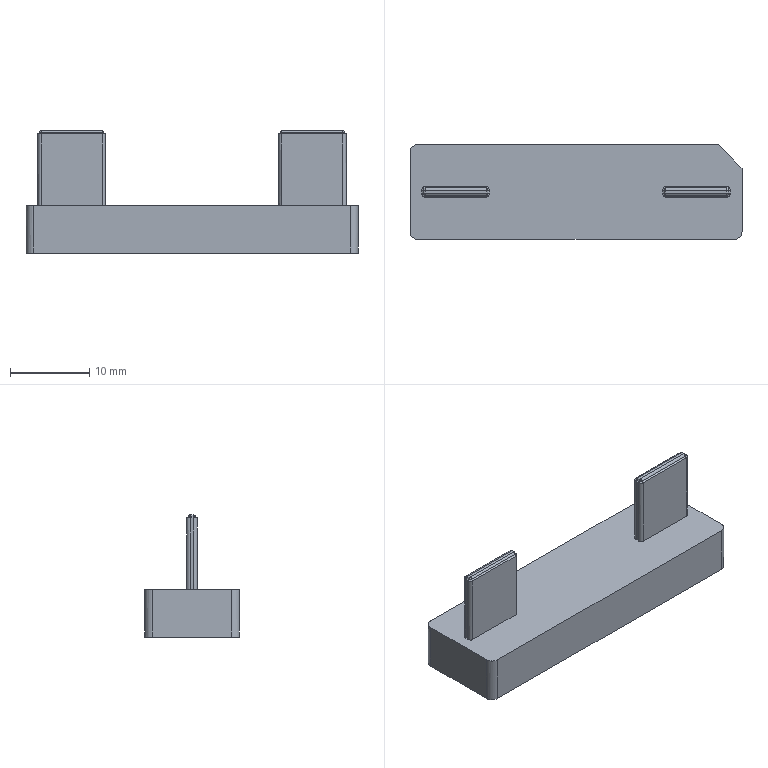NC program | PowerMill | posted with a generic post | part box 42 x 12 x 15.447 mm
Lines 10041 to 10905 of 88764:
N10138 M6
N10139 S18000 M03
N10140 G00 G90 X0.0 Y0.0
N10141 G43 Z10.797 H14
N10142
N10143 G05 P10000 R8
N10144 X20.3526 Y-2.564
N10145 Z0.922
N10146 G01 Z-0.278 F1200.0
N10147 X20.3332 Y-2.4952 F2000.0
N10148 X20.3063 Y-2.4291
N10149 X20.2722 Y-2.3663
N10150 X20.2313 Y-2.3077
N10151 X20.1841 Y-2.254
N10152 X20.1312 Y-2.2059
N10153 X20.0734 Y-2.1641
N10154 X20.0112 Y-2.1289
N10155 X19.9455 Y-2.1009
N10156 X19.877 Y-2.0804
N10157 X19.8067 Y-2.0676
N10158 X19.7354 Y-2.0628
N10159 X19.664 Y-2.0659
N10160 X19.5935 Y-2.077
N10161 X19.589 Y-2.078
N10162 X19.4691 Y-2.1046
N10163 X19.3617 Y-2.1219
N10164 X19.24 Y-2.1338
N10165 X19.1048 Y-2.1394
N10166 X18.6048 Y-2.1399
N10167 X18.1048
N10168 X17.6048 Y-2.14
N10169 X17.1048
N10170 X16.6048
N10171 X16.1048
N10172 X15.6048 Y-2.1399
N10173 X15.1129
N10174 X14.621
N10175 X14.1292
N10176 X13.6374 Y-2.14
N10177 X13.1456 Y-2.1401
N10178 X12.6538
N10179 X12.162 Y-2.1403
N10180 X11.6702 Y-2.1406
N10181 X11.4289 Y-2.1408
N10182 X11.2906 Y-2.1373
N10183 X11.1595 Y-2.1265
N10184 X11.0349 Y-2.1087
N10185 X10.9163 Y-2.0842
N10186 X10.8016 Y-2.0527
N10187 X10.6821 Y-2.0117
N10188 X10.5659 Y-1.9634
N10189 X10.4536 Y-1.9081
N10190 X10.3455 Y-1.846
N10191 X10.242 Y-1.7775
N10192 X10.1435 Y-1.7027
N10193 X10.0489 Y-1.6211
N10194 X9.96 Y-1.5341
N10195 X9.8771 Y-1.4418
N10196 X9.8 Y-1.3442
N10197 X9.7288 Y-1.2412
N10198 X9.6636 Y-1.1327
N10199 X9.6043 Y-1.0189
N10200 X9.5539 Y-0.906
N10201 X9.512 Y-0.7933
N10202 X9.4784 Y-0.6813
N10203 X9.4571 Y-0.5918
N10204 X9.4387 Y-0.5016
N10205 X9.4242 Y-0.4109
N10206 X9.4151 Y-0.3193
N10207 X9.4113 Y-0.2272
N10208 X9.4118 Y0.2682
N10209 X9.4163 Y0.3659
N10210 X9.4284 Y0.463
N10211 X9.445 Y0.5596
N10212 X9.4639 Y0.6555
N10213 X9.4927 Y0.764
N10214 X9.5308 Y0.8775
N10215 X9.5775 Y0.9928
N10216 X9.6318 Y1.1063
N10217 X9.6916 Y1.2136
N10218 X9.7586 Y1.3178
N10219 X9.8334 Y1.4194
N10220 X9.9148 Y1.5169
N10221 X10.0011 Y1.6081
N10222 X10.0918 Y1.6926
N10223 X10.187 Y1.7705
N10224 X10.2875 Y1.8424
N10225 X10.3927 Y1.9078
N10226 X10.5022 Y1.9666
N10227 X10.6156 Y2.0184
N10228 X10.7325 Y2.0629
N10229 X10.8518 Y2.0999
N10230 X10.961 Y2.1271
N10231 X11.0715 Y2.1479
N10232 X11.1832 Y2.1622
N10233 X11.3088 Y2.1706
N10234 X11.4243 Y2.1728
N10235 X11.9156
N10236 X12.4068
N10237 X12.8979
N10238 X13.3891
N10239 X13.8803
N10240 X14.3714
N10241 X14.8625
N10242 X15.3536 Y2.1727
N10243 X15.8446
N10244 X16.3357
N10245 X16.8267 Y2.1728
N10246 X17.3177 Y2.173
N10247 X17.8086 Y2.1731
N10248 X18.2995 Y2.1733
N10249 X18.7904 Y2.1736
N10250 X19.0484 Y2.1738
N10251 X19.1858 Y2.1703
N10252 X19.3171 Y2.1595
N10253 X19.4429 Y2.1415
N10254 X19.564 Y2.1164
N10255 X19.6819 Y2.0841
N10256 X19.7976 Y2.0442
N10257 X19.9139 Y1.9957
N10258 X20.0265 Y1.9401
N10259 X20.135 Y1.8777
N10260 X20.2389 Y1.8088
N10261 X20.3377 Y1.7337
N10262 X20.4314 Y1.6525
N10263 X20.5198 Y1.5655
N10264 X20.6038 Y1.4717
N10265 X20.682 Y1.3724
N10266 X20.7542 Y1.2679
N10267 X20.8199 Y1.1586
N10268 X20.8774 Y1.0478
N10269 X20.9282 Y0.9327
N10270 X20.9712 Y0.8154
N10271 X21.0062 Y0.6975
N10272 X21.0329 Y0.5802
N10273 X21.0526 Y0.4631
N10274 X21.0649 Y0.3501
N10275 X21.0694 Y0.2422
N10276 X21.0688 Y-0.1885
N10277 X21.0671 Y-0.2921
N10278 X21.0583 Y-0.3984
N10279 X21.0412 Y-0.5104
N10280 X21.0152 Y-0.6295
N10281 X20.9813 Y-0.751
N10282 X20.9401 Y-0.8698
N10283 X20.8914 Y-0.9858
N10284 X20.8355 Y-1.0985
N10285 X20.7726 Y-1.2075
N10286 X20.7028 Y-1.3124
N10287 X20.6264 Y-1.4127
N10288 X20.5438 Y-1.508
N10289 X20.4553 Y-1.5979
N10290 X20.3612 Y-1.6823
N10291 X20.2716 Y-1.7533
N10292 X20.1752 Y-1.8204
N10293 X20.0699 Y-1.8843
N10294 X19.9577 Y-1.9432
N10295 X19.8435 Y-1.9943
N10296 X19.7306 Y-2.0366
N10297 X19.6212 Y-2.0697
N10298 X19.589 Y-2.078
N10299 X19.4894 Y-2.1004
N10300 X19.3889 Y-2.1184
N10301 X19.2669 Y-2.1323 Z-0.2781
N10302 X19.1358 Y-2.1395
N10303 X18.6358 Y-2.1409 Z-0.2783
N10304 X18.1358 Y-2.1418 Z-0.2785
N10305 X17.6358 Y-2.143 Z-0.2787
N10306 X17.1358 Y-2.144 Z-0.2789
N10307 X16.6358 Y-2.1447 Z-0.2791
N10308 X16.1358 Y-2.1455 Z-0.2792
N10309 X15.6358 Y-2.1463 Z-0.2794
N10310 X15.1404 Y-2.147 Z-0.2796
N10311 X14.645 Y-2.1478 Z-0.2797
N10312 X14.1497 Y-2.1485 Z-0.2799
N10313 X13.6544 Y-2.1493 Z-0.28
N10314 X13.159 Y-2.1499 Z-0.2802
N10315 X12.6637 Y-2.1504 Z-0.2803
N10316 X12.1684 Y-2.1509 Z-0.2805
N10317 X11.6731 Y-2.152 Z-0.2806
N10318 X11.4289 Y-2.1529
N10319 X11.2951 Y-2.1498
N10320 X11.1628 Y-2.1395
N10321 X11.036 Y-2.1221
N10322 X10.9166 Y-2.0983
N10323 X10.8055 Y-2.0686 Z-0.2805
N10324 X10.7001 Y-2.0329
N10325 X10.5823 Y-1.9857
N10326 X10.4757 Y-1.9353 Z-0.2804
N10327 X10.3828 Y-1.8839
N10328 X10.298 Y-1.8316 Z-0.2805
N10329 X10.216 Y-1.7752 Z-0.2807
N10330 X10.1372 Y-1.7143 Z-0.2808
N10331 X10.0407 Y-1.6308
N10332 X9.9501 Y-1.5419 Z-0.2809
N10333 X9.8659 Y-1.4484
N10334 X9.7887 Y-1.3508 Z-0.281
N10335 X9.7188 Y-1.2497
N10336 X9.6619 Y-1.1563 Z-0.2811
N10337 X9.6029 Y-1.0465 Z-0.2813
N10338 X9.557 Y-0.9473 Z-0.2814
N10339 X9.5184 Y-0.849
N10340 X9.4776 Y-0.726
N10341 X9.445 Y-0.6031 Z-0.2815
N10342 X9.421 Y-0.484
N10343 X9.4057 Y-0.3706 Z-0.2816
N10344 X9.3985 Y-0.2638 Z-0.2817
N10345 X9.3962 Y0.2357
N10346 X9.4001 Y0.3396
N10347 X9.4107 Y0.4458 Z-0.2818
N10348 X9.4295 Y0.5633
N10349 X9.4573 Y0.689 Z-0.2819
N10350 X9.491 Y0.8076
N10351 X9.5278 Y0.9131 Z-0.282
N10352 X9.5699 Y1.0142
N10353 X9.6257 Y1.1291 Z-0.2819
N10354 X9.6896 Y1.2428
N10355 X9.7491 Y1.3348
N10356 X9.8198 Y1.4301
N10357 X9.8874 Y1.5125
N10358 X9.9581 Y1.5897 Z-0.282
N10359 X10.041 Y1.6703 Z-0.2823
N10360 X10.1199 Y1.7393 Z-0.2824
N10361 X10.2022 Y1.804
N10362 X10.3047 Y1.8752
N10363 X10.4118 Y1.94
N10364 X10.5233 Y1.998
N10365 X10.6388 Y2.0491 Z-0.2825
N10366 X10.7579 Y2.0931
N10367 X10.8801 Y2.13
N10368 X10.9978 Y2.1578
N10369 X11.1109 Y2.1769
N10370 X11.2202 Y2.1878
N10371 X11.3491 Y2.193 Z-0.2829
N10372 X11.8464 Y2.1942 Z-0.2833
N10373 X12.3437 Y2.195 Z-0.2835
N10374 X12.841 Y2.1958 Z-0.2836
N10375 X13.3383 Y2.1965 Z-0.2838
N10376 X13.8355 Y2.1971 Z-0.284
N10377 X14.3327 Y2.1977 Z-0.2841
N10378 X14.8299 Y2.1984 Z-0.2843
N10379 X15.3271 Y2.1992 Z-0.2845
N10380 X15.8242 Y2.1999 Z-0.2847
N10381 X16.3213 Y2.2006 Z-0.2849
N10382 X16.8184 Y2.2013 Z-0.2851
N10383 X17.3154 Y2.202 Z-0.2853
N10384 X17.8125 Y2.2028 Z-0.2854
N10385 X18.3095 Y2.2036 Z-0.2856
N10386 X18.8064 Y2.2045 Z-0.2857
N10387 X18.9732 Y2.2049
N10388 X19.0454 Y2.2051
N10389 X19.1176 Y2.2052
N10390 X19.1898 Y2.2044
N10391 X19.2619 Y2.2001 Z-0.2858
N10392 X19.3336 Y2.192
N10393 X19.4051 Y2.1823
N10394 X19.5208 Y2.161
N10395 X19.6387 Y2.1313
N10396 X19.7585 Y2.093 Z-0.2859
N10397 X19.8778 Y2.0469
N10398 X19.9912 Y1.9948 Z-0.286
N10399 X20.0927 Y1.9404 Z-0.2861
N10400 X20.1909 Y1.8799
N10401 X20.2937 Y1.8079 Z-0.2862
N10402 X20.3919 Y1.7299
N10403 X20.4781 Y1.6525 Z-0.2863
N10404 X20.5587 Y1.5703
N10405 X20.6421 Y1.4745 Z-0.2864
N10406 X20.7193 Y1.3737
N10407 X20.7903 Y1.2679 Z-0.2865
N10408 X20.8553 Y1.1568
N10409 X20.9089 Y1.0516 Z-0.2866
N10410 X20.9561 Y0.9435 Z-0.2867
N10411 X20.9974 Y0.8291
N10412 X21.033 Y0.7076 Z-0.2868
N10413 X21.0627 Y0.5782
N10414 X21.0809 Y0.4686 Z-0.2869
N10415 X21.0932 Y0.3479
N10416 X21.0999 Y0.2097
N10417 X21.1011 Y0.0391 Z-0.287
N10418 X21.099 Y-0.1874 Z-0.2871
N10419 X21.0979 Y-0.2647
N10420 X21.0938 Y-0.3419
N10421 X21.0852 Y-0.4187 Z-0.2872
N10422 X21.0722 Y-0.4951
N10423 X21.0582 Y-0.5712
N10424 X21.0426 Y-0.647
N10425 X21.016 Y-0.7433 Z-0.2873
N10426 X20.9761 Y-0.8621
N10427 X20.9295 Y-0.9782 Z-0.2874
N10428 X20.8754 Y-1.0917
N10429 X20.8135 Y-1.2028 Z-0.2875
N10430 X20.7439 Y-1.3117
N10431 X20.6749 Y-1.4071
N10432 X20.5994 Y-1.4987 Z-0.2876
N10433 X20.5146 Y-1.5895
N10434 X20.4278 Y-1.6724 Z-0.2877
N10435 X20.3357 Y-1.7504
N10436 X20.2363 Y-1.8241 Z-0.2878
N10437 X20.1306 Y-1.8927
N10438 X20.0198 Y-1.9551
N10439 X19.9058 Y-2.0102 Z-0.2879
N10440 X19.7907 Y-2.0571
N10441 X19.676 Y-2.0957 Z-0.288
N10442 X19.5985 Y-2.1172
N10443 X19.4951 Y-2.1417
N10444 X19.3904 Y-2.1599 Z-0.2881
N10445 X19.2848 Y-2.1724
N10446 X19.1751 Y-2.1792
N10447 X19.0483 Y-2.181 Z-0.2882
N10448 X18.5483 Y-2.1813 Z-0.2884
N10449 X18.0483 Y-2.1817 Z-0.2885
N10450 X17.5483 Y-2.1822 Z-0.2887
N10451 X17.0483 Y-2.1827 Z-0.2889
N10452 X16.5483 Y-2.1833 Z-0.2891
N10453 X16.0483 Y-2.1838 Z-0.2892
N10454 X15.5483 Y-2.1843 Z-0.2894
N10455 X15.0513 Y-2.1847 Z-0.2896
N10456 X14.5543 Y-2.1851 Z-0.2897
N10457 X14.0573 Y-2.1855 Z-0.2899
N10458 X13.5603 Y-2.186 Z-0.2901
N10459 X13.0633 Y-2.1864 Z-0.2903
N10460 X12.5664 Y-2.1868 Z-0.2904
N10461 X12.0694 Y-2.1873 Z-0.2906
N10462 X11.5725 Y-2.1882 Z-0.2908
N10463 X11.4272 Y-2.1886
N10464 X11.2915 Y-2.1859 Z-0.2909
N10465 X11.1735 Y-2.1771
N10466 X11.0592 Y-2.1618 Z-0.291
N10467 X10.9327 Y-2.1378
N10468 X10.8127 Y-2.1073 Z-0.2911
N10469 X10.6978 Y-2.0702
N10470 X10.5846 Y-2.0253
N10471 X10.4719 Y-1.9722
N10472 X10.3609 Y-1.911 Z-0.2912
N10473 X10.2533 Y-1.8426
N10474 X10.151 Y-1.7683 Z-0.2913
N10475 X10.0553 Y-1.6891 Z-0.2914
N10476 X9.9672 Y-1.6061
N10477 X9.8858 Y-1.5197
N10478 X9.8093 Y-1.429 Z-0.2915
N10479 X9.7382 Y-1.334
N10480 X9.6691 Y-1.2288 Z-0.2916
N10481 X9.6073 Y-1.1204
N10482 X9.5525 Y-1.0084
N10483 X9.5032 Y-0.8897 Z-0.2917
N10484 X9.4607 Y-0.7666
N10485 X9.4282 Y-0.6512 Z-0.2918
N10486 X9.4029 Y-0.5334
N10487 X9.3844 Y-0.4103 Z-0.2919
N10488 X9.3731 Y-0.2816
N10489 X9.3691 Y-0.1469 Z-0.292
N10490 X9.3699 Y-0.0057
N10491 X9.3684 Y0.1655 Z-0.2921
N10492 X9.3687 Y0.2557
N10493 X9.3738 Y0.3457
N10494 X9.3784 Y0.3887
N10495 X9.3834 Y0.4317 Z-0.2922
N10496 X9.3918 Y0.4976
N10497 X9.398 Y0.5404
N10498 X9.4057 Y0.5829
N10499 X9.4254 Y0.6742
N10500 X9.4459 Y0.7514 Z-0.2923
N10501 X9.485 Y0.876
N10502 X9.528 Y0.9893 Z-0.2924
N10503 X9.5768 Y1.0968
N10504 X9.6364 Y1.2091
N10505 X9.7031 Y1.3179 Z-0.2925
N10506 X9.7767 Y1.4225
N10507 X9.8565 Y1.5223 Z-0.2926
N10508 X9.9423 Y1.6166
N10509 X10.0333 Y1.705 Z-0.2927
N10510 X10.1292 Y1.7871
N10511 X10.2235 Y1.858
N10512 X10.3269 Y1.926 Z-0.2928
N10513 X10.4345 Y1.9885
N10514 X10.5456 Y2.0444 Z-0.2929
N10515 X10.6603 Y2.0932
N10516 X10.7785 Y2.1348 Z-0.293
N10517 X10.9001 Y2.1692
N10518 X11.0185 Y2.1953
N10519 X11.1297 Y2.2126
N10520 X11.2368 Y2.2218 Z-0.2931
N10521 X11.3709 Y2.2259
N10522 X11.87 Y2.2266 Z-0.2933
N10523 X12.3691 Y2.2268 Z-0.2934
N10524 X12.8682 Y2.2271 Z-0.2936
N10525 X13.3672 Y2.2275 Z-0.2937
N10526 X13.8663 Y2.2279 Z-0.2939
N10527 X14.3653 Y2.2283 Z-0.294
N10528 X14.8643 Y2.2287 Z-0.2942
N10529 X15.3632 Y2.2291 Z-0.2944
N10530 X15.8622 Y2.2295 Z-0.2945
N10531 X16.3611 Y2.2299 Z-0.2947
N10532 X16.8599 Y2.2304 Z-0.2949
N10533 X17.3588 Y2.2309 Z-0.2951
N10534 X17.8576 Y2.2314 Z-0.2953
N10535 X18.3564 Y2.2318 Z-0.2955
N10536 X18.8552 Y2.2327 Z-0.2957
N10537 X18.9907 Y2.2331 Z-0.2958
N10538 X19.1364 Y2.234 Z-0.2959
N10539 X19.2278 Y2.2313
N10540 X19.3189 Y2.2227
N10541 X19.4345 Y2.206 Z-0.296
N10542 X19.5492 Y2.1835
N10543 X19.6724 Y2.1516
N10544 X19.7912 Y2.1127 Z-0.2961
N10545 X19.9054 Y2.0672
N10546 X20.0151 Y2.0151 Z-0.2962
N10547 X20.1206 Y1.9564
N10548 X20.2258 Y1.8903 Z-0.2963
N10549 X20.3193 Y1.8232
N10550 X20.4154 Y1.7446
N10551 X20.5086 Y1.6582 Z-0.2964
N10552 X20.5971 Y1.5656
N10553 X20.6791 Y1.4686 Z-0.2965
N10554 X20.7545 Y1.3671
N10555 X20.8234 Y1.261 Z-0.2966
N10556 X20.8857 Y1.1503
N10557 X20.9409 Y1.0363
N10558 X20.9893 Y0.9186 Z-0.2967
N10559 X21.0312 Y0.7958
N10560 X21.0606 Y0.6917 Z-0.2968
N10561 X21.0835 Y0.5888
N10562 X21.1008 Y0.4849
N10563 X21.1117 Y0.3915 Z-0.2969
N10564 X21.1193 Y0.2977
N10565 X21.1211 Y0.2036
N10566 X21.1203 Y0.1095 Z-0.297
N10567 X21.1213 Y-0.0694
N10568 X21.1207 Y-0.1973 Z-0.2971
N10569 X21.1133 Y-0.3475
N10570 X21.1083 Y-0.3982 Z-0.2972
N10571 X21.1015 Y-0.4486
N10572 X21.0939 Y-0.499
N10573 X21.0856 Y-0.5492
N10574 X21.0758 Y-0.5992
N10575 X21.0475 Y-0.7125 Z-0.2973
N10576 X21.0096 Y-0.8352
N10577 X20.9682 Y-0.9465
N10578 X20.9183 Y-1.058 Z-0.2974
N10579 X20.8597 Y-1.1699
N10580 X20.7921 Y-1.282 Z-0.2975
N10581 X20.7215 Y-1.3848
N10582 X20.6439 Y-1.4837 Z-0.2976
N10583 X20.5595 Y-1.5784
N10584 X20.4687 Y-1.6683 Z-0.2977
N10585 X20.3729 Y-1.7521
N10586 X20.2731 Y-1.8289
N10587 X20.1696 Y-1.8986 Z-0.2978
N10588 X20.0626 Y-1.9612
N10589 X19.948 Y-2.0193 Z-0.2979
N10590 X19.834 Y-2.0685
N10591 X19.7208 Y-2.1092 Z-0.298
N10592 X19.6083 Y-2.1414
N10593 X19.6044 Y-2.1424
N10594 X19.5407 Y-2.158
N10595 X19.4763 Y-2.1713
N10596 X19.4117 Y-2.1829 Z-0.2981
N10597 X19.3468 Y-2.1925
N10598 X19.2815 Y-2.1992
N10599 X19.16 Y-2.206 Z-0.2982
N10600 X19.0061 Y-2.2077
N10601 X18.5061 Y-2.2072 Z-0.2984
N10602 X18.0061 Y-2.2082 Z-0.2986
N10603 X17.5061 Y-2.2088 Z-0.2987
N10604 X17.0061 Y-2.2092 Z-0.2989
N10605 X16.5061 Y-2.2097 Z-0.2991
N10606 X16.0061 Y-2.2101 Z-0.2992
N10607 X15.5061 Y-2.2106 Z-0.2994
N10608 X15.0074 Y-2.2111 Z-0.2996
N10609 X14.5088 Y-2.2115 Z-0.2998
N10610 X14.0102 Y-2.212 Z-0.2999
N10611 X13.5116 Y-2.2125 Z-0.3001
N10612 X13.013 Y-2.2128 Z-0.3003
N10613 X12.5144 Y-2.2131 Z-0.3004
N10614 X12.0158 Y-2.2137 Z-0.3006
N10615 X11.5172 Y-2.2148 Z-0.3008
N10616 X11.37 Y-2.2147
N10617 X11.2358 Y-2.2088 Z-0.3009
N10618 X11.1115 Y-2.1962
N10619 X10.9902 Y-2.1762 Z-0.301
N10620 X10.867 Y-2.148
N10621 X10.7445 Y-2.1117 Z-0.3011
N10622 X10.6278 Y-2.0691
N10623 X10.5137 Y-2.0189
N10624 X10.4028 Y-1.9614 Z-0.3012
N10625 X10.2955 Y-1.8972
N10626 X10.1894 Y-1.8251 Z-0.3013
N10627 X10.0912 Y-1.7491
N10628 X10.0005 Y-1.6693 Z-0.3014
N10629 X9.915 Y-1.5841
N10630 X9.8301 Y-1.4885
N10631 X9.7515 Y-1.388 Z-0.3015
N10632 X9.6793 Y-1.2828
N10633 X9.6125 Y-1.1721 Z-0.3016
N10634 X9.5545 Y-1.0611
N10635 X9.505 Y-0.95 Z-0.3017
N10636 X9.4628 Y-0.8368
N10637 X9.4242 Y-0.7116 Z-0.3018
N10638 X9.3936 Y-0.5858
N10639 X9.3711 Y-0.4599
N10640 X9.3566 Y-0.3344 Z-0.3019
N10641 X9.3501 Y-0.2092
N10642 X9.3491 Y-0.0455 Z-0.302
N10643 X9.3509 Y0.1966 Z-0.3021
N10644 X9.3551 Y0.3468
N10645 X9.3595 Y0.3983
N10646 X9.3653 Y0.4497 Z-0.3022
N10647 X9.3721 Y0.501
N10648 X9.3939 Y0.6227
N10649 X9.4241 Y0.7469 Z-0.3023
N10650 X9.4607 Y0.8665
N10651 X9.5052 Y0.9849
N10652 X9.5576 Y1.102 Z-0.3024
N10653 X9.6177 Y1.2164
N10654 X9.6842 Y1.3263 Z-0.3025
N10655 X9.7563 Y1.4302
N10656 X9.834 Y1.5285 Z-0.3026
N10657 X9.9191 Y1.6234
N10658 X10.01 Y1.7128 Z-0.3027
N10659 X10.1062 Y1.7963
N10660 X10.2074 Y1.8734
N10661 X10.3132 Y1.9441 Z-0.3028
N10662 X10.4231 Y2.008
N10663 X10.5379 Y2.0657 Z-0.3029
N10664 X10.6527 Y2.1149
N10665 X10.7675 Y2.1556 Z-0.303
N10666 X10.882 Y2.1881
N10667 X10.9966 Y2.2127
N10668 X11.121 Y2.2338 Z-0.3031
N10669 X11.2238 Y2.2454
N10670 X11.3169 Y2.2492
N10671 X11.8026 Y2.2502 Z-0.3033
N10672 X12.2883 Y2.2506 Z-0.3035
N10673 X12.7739 Y2.251 Z-0.3037
N10674 X13.2595 Y2.2514 Z-0.3038
N10675 X13.7452 Y2.2518 Z-0.304
N10676 X14.2307 Y2.2522 Z-0.3042
N10677 X14.7163 Y2.2526 Z-0.3043
N10678 X15.2019 Y2.253 Z-0.3045
N10679 X15.6874 Y2.2534 Z-0.3047
N10680 X16.1729 Y2.2538 Z-0.3048
N10681 X16.6583 Y2.2542 Z-0.305
N10682 X17.1438 Y2.2547 Z-0.3052
N10683 X17.6292 Y2.255 Z-0.3053
N10684 X18.1146 Y2.2553 Z-0.3055
N10685 X18.5999 Y2.2559 Z-0.3057
N10686 X19.0853 Y2.2574 Z-0.3058
N10687 X19.2219 Y2.2523 Z-0.3059
N10688 X19.3529 Y2.2399
N10689 X19.4785 Y2.2203 Z-0.306
N10690 X19.5988 Y2.1939
N10691 X19.7168 Y2.1601
N10692 X19.8364 Y2.1176 Z-0.3061
N10693 X19.9533 Y2.0677
N10694 X20.0671 Y2.0104 Z-0.3062
N10695 X20.1774 Y1.9459
N10696 X20.2831 Y1.875 Z-0.3063
N10697 X20.3822 Y1.7992
N10698 X20.4749 Y1.7186 Z-0.3064
N10699 X20.5668 Y1.6278
N10700 X20.6527 Y1.5319
N10701 X20.7322 Y1.4312 Z-0.3065
N10702 X20.8051 Y1.3259
N10703 X20.8711 Y1.2166 Z-0.3066
N10704 X20.9302 Y1.1034
N10705 X20.982 Y0.9868 Z-0.3067
N10706 X21.0266 Y0.8671
N10707 X21.0639 Y0.7446 Z-0.3068
N10708 X21.0945 Y0.6181
N10709 X21.1167 Y0.4943
N10710 X21.1306 Y0.3733 Z-0.3069
N10711 X21.1364 Y0.2551
N10712 X21.1374 Y0.1372 Z-0.307
N10713 X21.1392 Y-0.0808
N10714 X21.136 Y-0.2383 Z-0.3071
N10715 X21.1281 Y-0.3624
N10716 X21.113 Y-0.486 Z-0.3072
N10717 X21.0898 Y-0.6106
N10718 X21.0584 Y-0.7357 Z-0.3073
N10719 X21.0199 Y-0.8577
N10720 X20.974 Y-0.9772 Z-0.3074
N10721 X20.9207 Y-1.0936
N10722 X20.8602 Y-1.2066
N10723 X20.7927 Y-1.3158 Z-0.3075
N10724 X20.7186 Y-1.4205
N10725 X20.6381 Y-1.5203 Z-0.3076
N10726 X20.5517 Y-1.6148
N10727 X20.4601 Y-1.7033 Z-0.3077
N10728 X20.3639 Y-1.7852
N10729 X20.2635 Y-1.8603 Z-0.3078
N10730 X20.1593 Y-1.9283
N10731 X20.0514 Y-1.9895
N10732 X19.9347 Y-2.0472 Z-0.3079
N10733 X19.8206 Y-2.0954
N10734 X19.7087 Y-2.1346 Z-0.308
N10735 X19.6091 Y-2.1625
N10736 X19.4962 Y-2.1884
N10737 X19.3751 Y-2.2083 Z-0.3081
N10738 X19.2514 Y-2.2209
N10739 X19.116 Y-2.2272 Z-0.3082
N10740 X18.616 Y-2.2282 Z-0.3083
N10741 X18.116 Y-2.2286 Z-0.3085
N10742 X17.616 Y-2.2288 Z-0.3087
N10743 X17.116 Y-2.229 Z-0.3089
N10744 X16.616 Y-2.2292 Z-0.309
N10745 X16.116 Y-2.2296 Z-0.3092
N10746 X15.616 Y-2.23 Z-0.3094
N10747 X15.116 Y-2.2303 Z-0.3095
N10748 X14.6232 Y-2.2305 Z-0.3097
N10749 X14.1304 Y-2.2309 Z-0.3099
N10750 X13.6375 Y-2.2312 Z-0.3101
N10751 X13.1447 Y-2.2315 Z-0.3102
N10752 X12.6519 Y-2.2318 Z-0.3104
N10753 X12.1592 Y-2.232 Z-0.3106
N10754 X11.6664 Y-2.2323 Z-0.3107
N10755 X11.429 Y-2.2326 Z-0.3108
N10756 X11.2845 Y-2.2294 Z-0.3109
N10757 X11.1543 Y-2.2197
N10758 X11.0348 Y-2.2036
N10759 X10.9235 Y-2.1814 Z-0.311
N10760 X10.8136 Y-2.1527
N10761 X10.6933 Y-2.114 Z-0.3111
N10762 X10.5767 Y-2.0684
N10763 X10.4638 Y-2.0158 Z-0.3112
N10764 X10.3546 Y-1.9561
N10765 X10.2487 Y-1.8895
N10766 X10.1471 Y-1.817 Z-0.3113
N10767 X10.0504 Y-1.7388
N10768 X9.9599 Y-1.6555 Z-0.3114
N10769 X9.8752 Y-1.5669
N10770 X9.7902 Y-1.4669 Z-0.3115
N10771 X9.7126 Y-1.3636
N10772 X9.6433 Y-1.2585
N10773 X9.5825 Y-1.1523 Z-0.3116
N10774 X9.5284 Y-1.0432
N10775 X9.4783 Y-0.9258 Z-0.3117
N10776 X9.4356 Y-0.8061
N10777 X9.4004 Y-0.6838 Z-0.3118
N10778 X9.3726 Y-0.5587
N10779 X9.3523 Y-0.4304
N10780 X9.3394 Y-0.2987 Z-0.3119
N10781 X9.3349 Y-0.2072
N10782 X9.3352 Y-0.1043 Z-0.312
N10783 X9.3354 Y0.0231
N10784 X9.3351 Y0.2311 Z-0.3121
N10785 X9.3395 Y0.3439
N10786 X9.3518 Y0.4651 Z-0.3122
N10787 X9.3724 Y0.5931
N10788 X9.4007 Y0.7195
N10789 X9.4368 Y0.844 Z-0.3123
N10790 X9.4804 Y0.9659
N10791 X9.5314 Y1.0846 Z-0.3124
N10792 X9.5894 Y1.1995
N10793 X9.6542 Y1.3103 Z-0.3125
N10794 X9.7255 Y1.4165
N10795 X9.8031 Y1.5178 Z-0.3126
N10796 X9.8826 Y1.6098
N10797 X9.9675 Y1.6975
N10798 X10.059 Y1.781 Z-0.3127
N10799 X10.1542 Y1.8575
N10800 X10.2528 Y1.9275 Z-0.3128
N10801 X10.3557 Y1.9921
N10802 X10.4644 Y2.051
N10803 X10.5793 Y2.1043 Z-0.3129
N10804 X10.7004 Y2.1517
N10805 X10.8192 Y2.1905 Z-0.313
N10806 X10.9304 Y2.2195
N10807 X11.04 Y2.2404 Z-0.3131
N10808 X11.1642 Y2.2566
N10809 X11.2974 Y2.2662
N10810 X11.429 Y2.269 Z-0.3132
N10811 X11.9124 Y2.2694 Z-0.3134
N10812 X12.3958 Y2.2697 Z-0.3135
N10813 X12.8791 Y2.2699 Z-0.3137
N10814 X13.3625 Y2.27 Z-0.3139
N10815 X13.8458 Y2.2703 Z-0.314
N10816 X14.3291 Y2.2706 Z-0.3142
N10817 X14.8124 Y2.2709 Z-0.3144
N10818 X15.2956 Y2.2711 Z-0.3145
N10819 X15.7789 Y2.2713 Z-0.3147
N10820 X16.2621 Y2.2715 Z-0.3149
N10821 X16.7453 Y2.2718 Z-0.315
N10822 X17.2284 Y2.2721 Z-0.3152
N10823 X17.7115 Y2.2724 Z-0.3153
N10824 X18.1946 Y2.2728 Z-0.3155
N10825 X18.6777 Y2.2731 Z-0.3157
N10826 X19.1607 Y2.2719 Z-0.3158
N10827 X19.2716 Y2.267 Z-0.3159
N10828 X19.3885 Y2.2542
N10829 X19.5106 Y2.2329 Z-0.316
N10830 X19.6296 Y2.2046
N10831 X19.7512 Y2.1677 Z-0.3161
N10832 X19.8703 Y2.1232
N10833 X19.9865 Y2.0712
N10834 X20.0995 Y2.012 Z-0.3162
N10835 X20.2088 Y1.9457
N10836 X20.3141 Y1.8725 Z-0.3163
N10837 X20.4147 Y1.7928
N10838 X20.5102 Y1.707 Z-0.3164
N10839 X20.6003 Y1.6153
N10840 X20.6838 Y1.5191
N10841 X20.7613 Y1.4176 Z-0.3165
N10842 X20.8327 Y1.3109
N10843 X20.8976 Y1.1996 Z-0.3166
N10844 X20.9542 Y1.0871
N10845 X21.0042 Y0.9703 Z-0.3167
N10846 X21.0479 Y0.8481
N10847 X21.0851 Y0.7206 Z-0.3168
N10848 X21.1128 Y0.603
N10849 X21.1294 Y0.5087
N10850 X21.1385 Y0.4221 Z-0.3169
N10851 X21.148 Y0.2982
N10852 X21.1509 Y0.1741
N10853 X21.151 Y0.0498 Z-0.317
N10854 Y-0.1155
N10855 X21.1486 Y-0.2636 Z-0.3171
N10856 X21.1407 Y-0.3855
N10857 X21.1274 Y-0.492 Z-0.3172
N10858 X21.1076 Y-0.5976
N10859 X21.0762 Y-0.7258 Z-0.3173
N10860 X21.0373 Y-0.8514
N10861 X20.9911 Y-0.9738
N10862 X20.9377 Y-1.0926 Z-0.3174
N10863 X20.8799 Y-1.2029
N10864 X20.8151 Y-1.3099 Z-0.3175
N10865 X20.7426 Y-1.4141
N10866 X20.6627 Y-1.5151 Z-0.3176
N10867 X20.5756 Y-1.6125
N10868 X20.4852 Y-1.702 Z-0.3177
N10869 X20.3904 Y-1.7849
N10870 X20.2917 Y-1.8607
N10871 X20.1893 Y-1.9294 Z-0.3178
N10872 X20.0815 Y-1.993
N10873 X19.9701 Y-2.0503 Z-0.3179
N10874 X19.8558 Y-2.1003
N10875 X19.7401 Y-2.1424 Z-0.318
N10876 X19.6231 Y-2.1773
N10877 X19.6134 Y-2.1799
N10878 X19.5264 Y-2.2006
N10879 X19.487 Y-2.2089
N10880 X19.4473 Y-2.2157 Z-0.3181
N10881 X19.3993 Y-2.2232
N10882 X19.3594 Y-2.229
N10883 X19.3195 Y-2.2342
N10884 X19.2795 Y-2.2384
N10885 X19.2393 Y-2.2415
N10886 X19.1737 Y-2.2456 Z-0.3182
N10887 X18.6737 Y-2.2461 Z-0.3183
N10888 X18.1737 Y-2.2464 Z-0.3185
N10889 X17.6737 Y-2.2467 Z-0.3187
N10890 X17.1737 Y-2.247 Z-0.3188
N10891 X16.6737 Y-2.2473 Z-0.319
N10892 X16.1737 Y-2.2476 Z-0.3192
N10893 X15.6737 Y-2.2479 Z-0.3194
N10894 X15.1737 Y-2.2482 Z-0.3195
N10895 X14.678 Y-2.2486 Z-0.3197
N10896 X14.1822 Y-2.2489 Z-0.3199
N10897 X13.6865 Y-2.2492 Z-0.32
N10898 X13.1908 Y-2.2495 Z-0.3202
N10899 X12.6951 Y-2.2497 Z-0.3204
N10900 X12.1994 Y-2.2499 Z-0.3205
N10901 X11.7037 Y-2.2502 Z-0.3207
N10902 X11.4272 Y-2.2505 Z-0.3208
N10903 X11.2843 Y-2.2473 Z-0.3209
N10904 X11.1545 Y-2.2374
N10905 X11.0346 Y-2.2212
N10906 X10.9229 Y-2.1987 Z-0.321
N10907 X10.8127 Y-2.1697
N10908 X10.6921 Y-2.1309 Z-0.3211
N10909 X10.5775 Y-2.0861
N10910 X10.4637 Y-2.033
N10911 X10.3514 Y-1.972 Z-0.3212
N10912 X10.2421 Y-1.9034
N10913 X10.1373 Y-1.8284 Z-0.3213
N10914 X10.0384 Y-1.7478
N10915 X9.9462 Y-1.6627 Z-0.3214
N10916 X9.86 Y-1.5724
N10917 X9.7767 Y-1.474 Z-0.3215
N10918 X9.6991 Y-1.3698
N10919 X9.6287 Y-1.2622
N10920 X9.5658 Y-1.1516 Z-0.3216
N10921 X9.5105 Y-1.0386
N10922 X9.4629 Y-0.9233 Z-0.3217
N10923 X9.419 Y-0.796
N10924 X9.3828 Y-0.6668 Z-0.3218
N10925 X9.358 Y-0.5545
N10926 X9.34 Y-0.4399
N10927 X9.3282 Y-0.3152 Z-0.3219
N10928 X9.3227 Y-0.177
N10929 X9.3224 Y-0.0181 Z-0.322
N10930 X9.3226 Y0.141
N10931 X9.3255 Y0.3 Z-0.3221
N10932 X9.3304 Y0.3907
N10933 X9.3421 Y0.4881 Z-0.3222
N10934 X9.3571 Y0.5842
N10935 X9.3698 Y0.6475
N10936 X9.3851 Y0.7104
N10937 X9.4076 Y0.7929 Z-0.3223
N10938 X9.4262 Y0.8549
N10939 X9.4469 Y0.9161
N10940 X9.4702 Y0.9764
N10941 X9.5229 Y1.0985 Z-0.3224
N10942 X9.5793 Y1.2107
N10943 X9.6426 Y1.3191 Z-0.3225
N10944 X9.7134 Y1.4247
N10945 X9.7921 Y1.528 Z-0.3226
N10946 X9.8728 Y1.6217
N10947 X9.9606 Y1.7116
N10948 X10.0557 Y1.7975 Z-0.3227
N10949 X10.1569 Y1.8784
N10950 X10.2626 Y1.9526 Z-0.3228
N10951 X10.371 Y2.0192
N10952 X10.4795 Y2.0769 Z-0.3229
N10953 X10.5913 Y2.1277
N10954 X10.7095 Y2.1726
N10955 X10.8307 Y2.2103 Z-0.323
N10956 X10.9508 Y2.2396
N10957 X11.0486 Y2.2581 Z-0.3231
N10958 X11.147 Y2.2721
N10959 X11.2461 Y2.2809
N10960 X11.3456 Y2.2849 Z-0.3232
N10961 X11.8334 Y2.286 Z-0.3233
N10962 X12.3211 Y2.2861 Z-0.3235
N10963 X12.8087 Z-0.3237
N10964 X13.2963 Z-0.3238
N10965 X13.7839 Y2.2863 Z-0.324
N10966 X14.2715 Y2.2866 Z-0.3242
N10967 X14.7591 Y2.2868 Z-0.3243
N10968 X15.2466 Y2.287 Z-0.3245
N10969 X15.7341 Y2.2872 Z-0.3247
N10970 X16.2216 Y2.2875 Z-0.3248
N10971 X16.7091 Y2.2877 Z-0.325
N10972 X17.1965 Y2.288 Z-0.3252
N10973 X17.6839 Y2.2884 Z-0.3253
N10974 X18.1713 Y2.2886 Z-0.3255
N10975 X18.6586 Y2.2889 Z-0.3257
N10976 X19.1459 Y2.2892 Z-0.3258
N10977 X19.2155 Y2.2876 Z-0.3259
N10978 X19.2848 Y2.282
N10979 X19.3606 Y2.2729
N10980 X19.4684 Y2.256
N10981 X19.5511 Y2.2399 Z-0.326
N10982 X19.6188 Y2.2239
N10983 X19.6858 Y2.2049
N10984 X19.8044 Y2.1649 Z-0.3261
N10985 X19.9266 Y2.1154
N10986 X20.0326 Y2.0657
N10987 X20.1367 Y2.0086 Z-0.3262
N10988 X20.2417 Y1.9423
N10989 X20.3458 Y1.8671 Z-0.3263
N10990 X20.4469 Y1.7844
N10991 X20.5415 Y1.6969 Z-0.3264
N10992 X20.6278 Y1.6067
N10993 X20.7048 Y1.5156
N10994 X20.7748 Y1.4218 Z-0.3265
N10995 X20.8462 Y1.3134
N10996 X20.9119 Y1.1992 Z-0.3266
N10997 X20.9719 Y1.0791
N10998 X21.0104 Y0.9914 Z-0.3267
N10999 X21.0339 Y0.929
N11000 X21.0551 Y0.8658
N11001 X21.0775 Y0.793
N11002 X21.1014 Y0.707 Z-0.3268